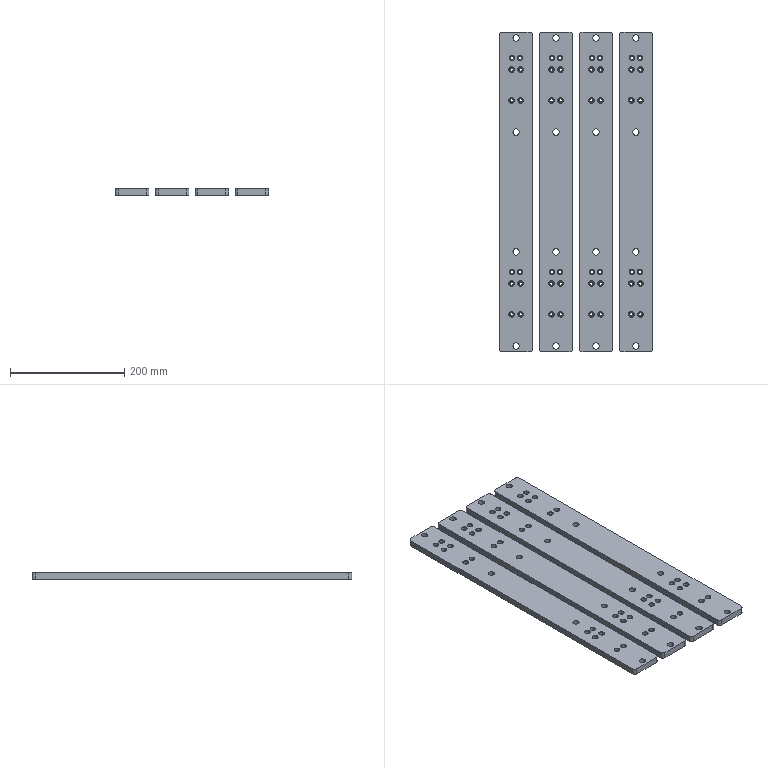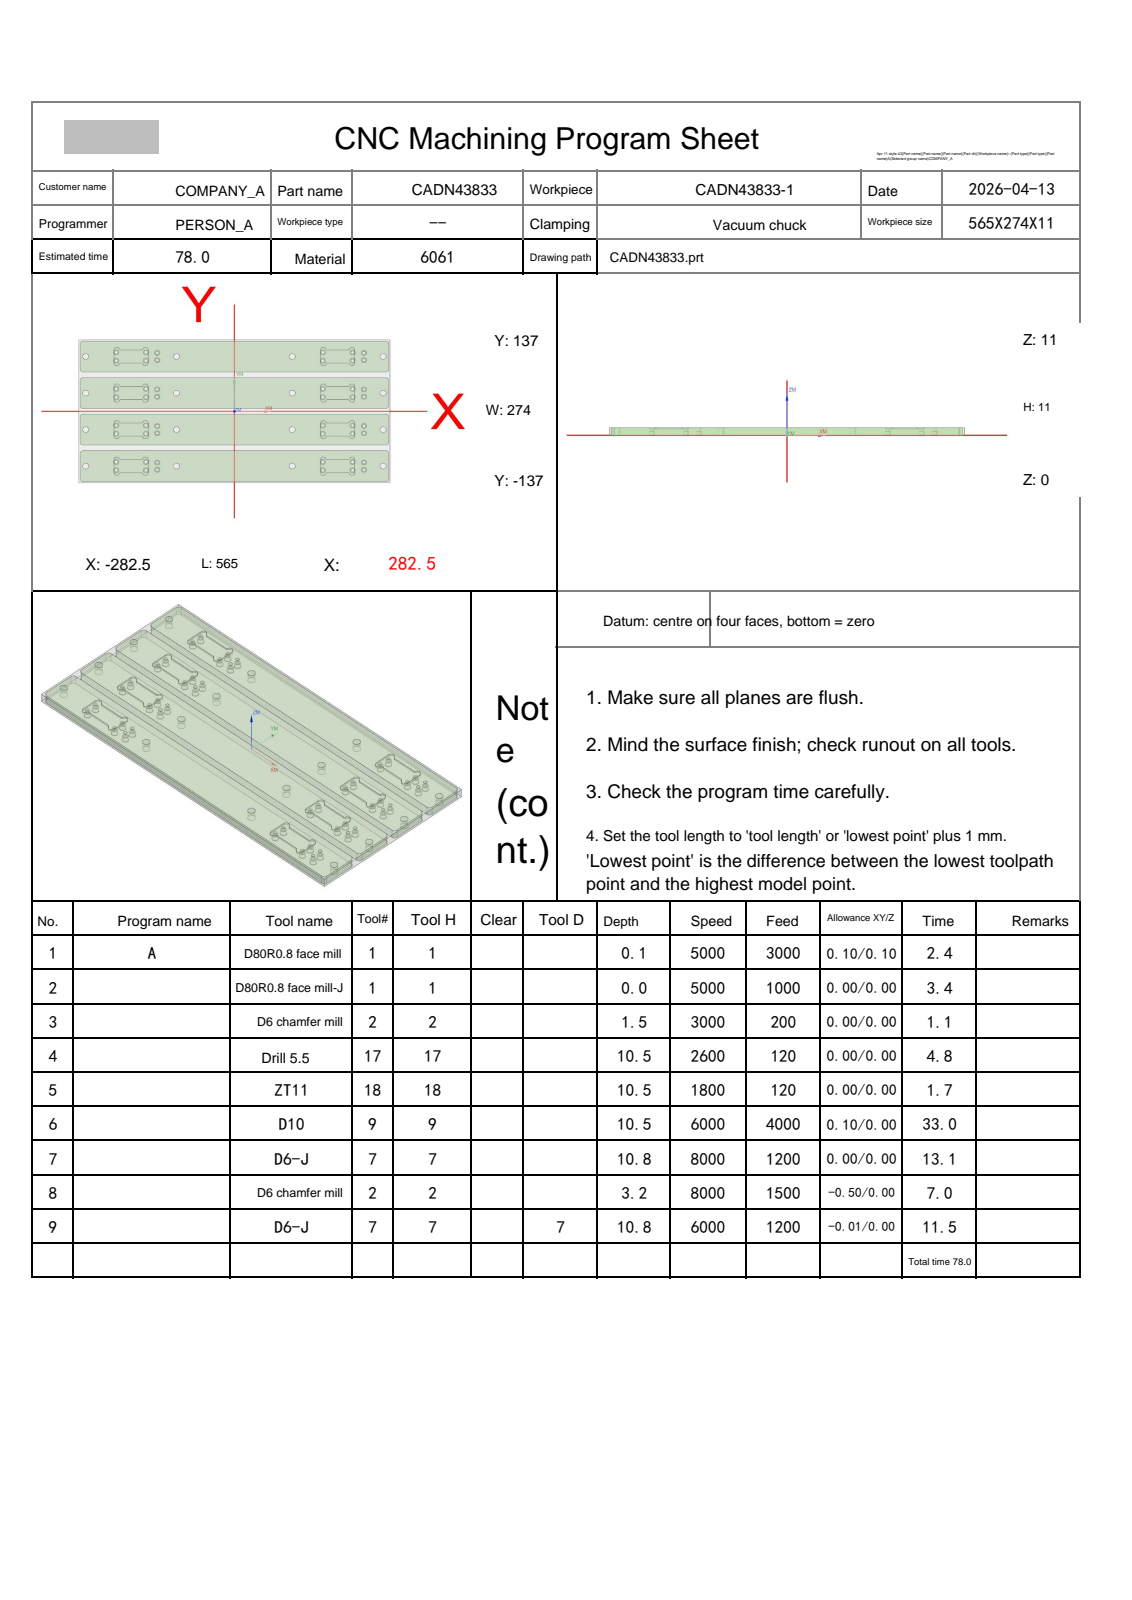NC program | NX | posted by the shop | part box 269 x 560 x 11 mm
Lines 4511 to 6644 of 6644, first 1747 of 2134 lines:
N8 T02 M06
(D6 chamfer mill  D=6. R=0. H=02 ce=0.00 di=0.00)
G00 G90 G54 X.386 Y74.373 M03 S8000
G43 H02 Z31.
M08
Z11.272
G01 Z9.8 F1350.
G03 X.1 Y74.573 I-1.286 J-1.532
G01 X.054 Y74.603
X0.0 Y74.6
X-275. F1500.
G02 X-280.9 Y80.5 I0.0 J5.9
G01 Y129.5
G02 X-275. Y135.4 I5.9 J0.0
G01 X275.
G02 X280.9 Y129.5 I0.0 J-5.9
G01 Y80.5
G02 X275. Y74.6 I-5.9 J0.0
G01 X0.0
X-.054 Y74.603
X-.1 Y74.573
G03 X-.386 Y74.373 I1. J-1.732
G01 Z11.272
G00 Z21.
X-269.6 Y109.399
Z11.323
G01 Z9.8 F1350.
G03 X-269.898 Y109.58 I-1.183 J-1.613
G01 X-269.946 Y109.606
X-270. Y109.6
G03 X-274.6 Y105. I0.0 J-4.6 F1500.
X-270. Y100.4 I4.6 J0.0
X-265.4 Y105. I0.0 J4.6
X-270. Y109.6 I-4.6 J0.0
G01 X-270.054 Y109.606
X-270.102 Y109.58
G03 X-270.4 Y109.399 I.885 J-1.794
G01 Z11.323
G00 Z21.
X-187.886 Y93.577
Z11.272
G01 Z9.8 F1350.
G03 X-187.6 Y93.377 I1.286 J1.532
G01 X-187.554 Y93.347
X-187.5 Y93.35
X-168.208 F1500.
G02 X-165.477 Y91.314 I0.0 J-2.85
G03 X-161.5 Y88.35 I3.977 J1.186
X-157.35 Y92.5 I0.0 J4.15
G01 Y117.5
G03 X-161.5 Y121.65 I-4.15 J0.0
X-165.477 Y118.686 I0.0 J-4.15
G02 X-168.208 Y116.65 I-2.731 J.814
G01 X-206.792
G02 X-209.523 Y118.686 I0.0 J2.85
G03 X-213.5 Y121.65 I-3.977 J-1.186
X-217.65 Y117.5 I0.0 J-4.15
G01 Y92.5
G03 X-213.5 Y88.35 I4.15 J0.0
X-209.523 Y91.314 I0.0 J4.15
G02 X-206.792 Y93.35 I2.731 J-.814
G01 X-187.5
X-187.446 Y93.347
X-187.4 Y93.377
G03 X-187.114 Y93.577 I-1. J1.732
G01 Z11.272
G00 Z21.
X-139.596 Y113.658
Z11.365
G01 Z9.8 F1350.
G03 X-139.898 Y113.832 I-1.147 J-1.638
G01 X-139.946 Y113.858
X-140. Y113.85
G03 X-141.85 Y112. I0.0 J-1.85 F1500.
X-140. Y110.15 I1.85 J0.0
X-138.15 Y112. I0.0 J1.85
X-139.679 Y113.822 I-1.85 J0.0
G01 X-140. Y113.85
X-140.054 Y113.858
X-140.102 Y113.832
G03 X-140.404 Y113.658 I.845 J-1.813
G01 Z11.365
G00 Z21.
X-139.596 Y99.658
Z11.365
G01 Z9.8 F1350.
G03 X-139.898 Y99.832 I-1.147 J-1.638
G01 X-139.946 Y99.858
X-140. Y99.85
G03 X-141.85 Y98. I0.0 J-1.85 F1500.
X-140. Y96.15 I1.85 J0.0
X-138.15 Y98. I0.0 J1.85
X-139.679 Y99.822 I-1.85 J0.0
G01 X-140. Y99.85
X-140.054 Y99.858
X-140.102 Y99.832
G03 X-140.404 Y99.658 I.845 J-1.813
G01 Z11.365
G00 Z21.
X-104.6 Y109.399
Z11.323
G01 Z9.8 F1350.
G03 X-104.898 Y109.58 I-1.183 J-1.613
G01 X-104.946 Y109.606
X-105. Y109.6
G03 X-109.6 Y105. I0.0 J-4.6 F1500.
X-105. Y100.4 I4.6 J0.0
X-100.4 Y105. I0.0 J4.6
X-105. Y109.6 I-4.6 J0.0
G01 X-105.054 Y109.606
X-105.102 Y109.58
G03 X-105.4 Y109.399 I.885 J-1.794
G01 Z11.323
G00 Z21.
X105.4
Z11.323
G01 Z9.8 F1350.
G03 X105.102 Y109.58 I-1.183 J-1.613
G01 X105.054 Y109.606
X105. Y109.6
G03 X100.4 Y105. I0.0 J-4.6 F1500.
X105. Y100.4 I4.6 J0.0
X109.6 Y105. I0.0 J4.6
X105. Y109.6 I-4.6 J0.0
G01 X104.946 Y109.606
X104.898 Y109.58
G03 X104.6 Y109.399 I.885 J-1.794
G01 Z11.323
G00 Z21.
X187.114 Y93.577
Z11.272
G01 Z9.8 F1350.
G03 X187.4 Y93.377 I1.286 J1.532
G01 X187.446 Y93.347
X187.5 Y93.35
X206.792 F1500.
G02 X209.523 Y91.314 I0.0 J-2.85
G03 X213.5 Y88.35 I3.977 J1.186
X217.65 Y92.5 I0.0 J4.15
G01 Y117.5
G03 X213.5 Y121.65 I-4.15 J0.0
X209.523 Y118.686 I0.0 J-4.15
G02 X206.792 Y116.65 I-2.731 J.814
G01 X168.208
G02 X165.477 Y118.686 I0.0 J2.85
G03 X161.5 Y121.65 I-3.977 J-1.186
X157.35 Y117.5 I0.0 J-4.15
G01 Y92.5
G03 X161.5 Y88.35 I4.15 J0.0
X165.477 Y91.314 I0.0 J4.15
G02 X168.208 Y93.35 I2.731 J-.814
G01 X187.5
X187.554 Y93.347
X187.6 Y93.377
G03 X187.886 Y93.577 I-1. J1.732
G01 Z11.272
G00 Z21.
X235.404 Y99.658
Z11.365
G01 Z9.8 F1350.
G03 X235.102 Y99.832 I-1.147 J-1.638
G01 X235.054 Y99.858
X235. Y99.85
G03 X233.15 Y98. I0.0 J-1.85 F1500.
X235. Y96.15 I1.85 J0.0
X236.85 Y98. I0.0 J1.85
X235.321 Y99.822 I-1.85 J0.0
G01 X235. Y99.85
X234.946 Y99.858
X234.898 Y99.832
G03 X234.596 Y99.658 I.845 J-1.813
G01 Z11.365
G00 Z21.
X235.404 Y113.658
Z11.365
G01 Z9.8 F1350.
G03 X235.102 Y113.832 I-1.147 J-1.638
G01 X235.054 Y113.858
X235. Y113.85
G03 X233.15 Y112. I0.0 J-1.85 F1500.
X235. Y110.15 I1.85 J0.0
X236.85 Y112. I0.0 J1.85
X235.321 Y113.822 I-1.85 J0.0
G01 X235. Y113.85
X234.946 Y113.858
X234.898 Y113.832
G03 X234.596 Y113.658 I.845 J-1.813
G01 Z11.365
G00 Z21.
X270.4 Y109.399
Z11.323
G01 Z9.8 F1350.
G03 X270.102 Y109.58 I-1.183 J-1.613
G01 X270.054 Y109.606
X270. Y109.6
G03 X265.4 Y105. I0.0 J-4.6 F1500.
X270. Y100.4 I4.6 J0.0
X274.6 Y105. I0.0 J4.6
X270. Y109.6 I-4.6 J0.0
G01 X269.946 Y109.606
X269.898 Y109.58
G03 X269.6 Y109.399 I.885 J-1.794
G01 Z11.323
G00 Z21.
X.386 Y4.373
Z11.272
G01 Z9.8 F1350.
G03 X.1 Y4.573 I-1.286 J-1.532
G01 X.054 Y4.603
X0.0 Y4.6
X-275. F1500.
G02 X-280.9 Y10.5 I0.0 J5.9
G01 Y59.5
G02 X-275. Y65.4 I5.9 J0.0
G01 X275.
G02 X280.9 Y59.5 I0.0 J-5.9
G01 Y10.5
G02 X275. Y4.6 I-5.9 J0.0
G01 X0.0
X-.054 Y4.603
X-.1 Y4.573
G03 X-.386 Y4.373 I1. J-1.732
G01 Z11.272
G00 Z21.
X-269.6 Y39.399
Z11.323
G01 Z9.8 F1350.
G03 X-269.898 Y39.58 I-1.183 J-1.613
G01 X-269.946 Y39.606
X-270. Y39.6
G03 X-274.6 Y35. I0.0 J-4.6 F1500.
X-270. Y30.4 I4.6 J0.0
X-265.4 Y35. I0.0 J4.6
X-270. Y39.6 I-4.6 J0.0
G01 X-270.054 Y39.606
X-270.102 Y39.58
G03 X-270.4 Y39.399 I.885 J-1.794
G01 Z11.323
G00 Z21.
X-187.886 Y23.577
Z11.272
G01 Z9.8 F1350.
G03 X-187.6 Y23.377 I1.286 J1.532
G01 X-187.554 Y23.347
X-187.5 Y23.35
X-168.208 F1500.
G02 X-165.477 Y21.314 I0.0 J-2.85
G03 X-161.5 Y18.35 I3.977 J1.186
X-157.35 Y22.5 I0.0 J4.15
G01 Y47.5
G03 X-161.5 Y51.65 I-4.15 J0.0
X-165.477 Y48.686 I0.0 J-4.15
G02 X-168.208 Y46.65 I-2.731 J.814
G01 X-206.792
G02 X-209.523 Y48.686 I0.0 J2.85
G03 X-213.5 Y51.65 I-3.977 J-1.186
X-217.65 Y47.5 I0.0 J-4.15
G01 Y22.5
G03 X-213.5 Y18.35 I4.15 J0.0
X-209.523 Y21.314 I0.0 J4.15
G02 X-206.792 Y23.35 I2.731 J-.814
G01 X-187.5
X-187.446 Y23.347
X-187.4 Y23.377
G03 X-187.114 Y23.577 I-1. J1.732
G01 Z11.272
G00 Z21.
X-139.596 Y29.658
Z11.365
G01 Z9.8 F1350.
G03 X-139.898 Y29.832 I-1.147 J-1.638
G01 X-139.946 Y29.858
X-140. Y29.85
G03 X-141.85 Y28. I0.0 J-1.85 F1500.
X-140. Y26.15 I1.85 J0.0
X-138.15 Y28. I0.0 J1.85
X-139.679 Y29.822 I-1.85 J0.0
G01 X-140. Y29.85
X-140.054 Y29.858
X-140.102 Y29.832
G03 X-140.404 Y29.658 I.845 J-1.813
G01 Z11.365
G00 Z21.
X-139.596 Y43.658
Z11.365
G01 Z9.8 F1350.
G03 X-139.898 Y43.832 I-1.147 J-1.638
G01 X-139.946 Y43.858
X-140. Y43.85
G03 X-141.85 Y42. I0.0 J-1.85 F1500.
X-140. Y40.15 I1.85 J0.0
X-138.15 Y42. I0.0 J1.85
X-139.679 Y43.822 I-1.85 J0.0
G01 X-140. Y43.85
X-140.054 Y43.858
X-140.102 Y43.832
G03 X-140.404 Y43.658 I.845 J-1.813
G01 Z11.365
G00 Z21.
X-104.6 Y39.399
Z11.323
G01 Z9.8 F1350.
G03 X-104.898 Y39.58 I-1.183 J-1.613
G01 X-104.946 Y39.606
X-105. Y39.6
G03 X-109.6 Y35. I0.0 J-4.6 F1500.
X-105. Y30.4 I4.6 J0.0
X-100.4 Y35. I0.0 J4.6
X-105. Y39.6 I-4.6 J0.0
G01 X-105.054 Y39.606
X-105.102 Y39.58
G03 X-105.4 Y39.399 I.885 J-1.794
G01 Z11.323
G00 Z21.
X105.4
Z11.323
G01 Z9.8 F1350.
G03 X105.102 Y39.58 I-1.183 J-1.613
G01 X105.054 Y39.606
X105. Y39.6
G03 X100.4 Y35. I0.0 J-4.6 F1500.
X105. Y30.4 I4.6 J0.0
X109.6 Y35. I0.0 J4.6
X105. Y39.6 I-4.6 J0.0
G01 X104.946 Y39.606
X104.898 Y39.58
G03 X104.6 Y39.399 I.885 J-1.794
G01 Z11.323
G00 Z21.
X187.114 Y23.577
Z11.272
G01 Z9.8 F1350.
G03 X187.4 Y23.377 I1.286 J1.532
G01 X187.446 Y23.347
X187.5 Y23.35
X206.792 F1500.
G02 X209.523 Y21.314 I0.0 J-2.85
G03 X213.5 Y18.35 I3.977 J1.186
X217.65 Y22.5 I0.0 J4.15
G01 Y47.5
G03 X213.5 Y51.65 I-4.15 J0.0
X209.523 Y48.686 I0.0 J-4.15
G02 X206.792 Y46.65 I-2.731 J.814
G01 X168.208
G02 X165.477 Y48.686 I0.0 J2.85
G03 X161.5 Y51.65 I-3.977 J-1.186
X157.35 Y47.5 I0.0 J-4.15
G01 Y22.5
G03 X161.5 Y18.35 I4.15 J0.0
X165.477 Y21.314 I0.0 J4.15
G02 X168.208 Y23.35 I2.731 J-.814
G01 X187.5
X187.554 Y23.347
X187.6 Y23.377
G03 X187.886 Y23.577 I-1. J1.732
G01 Z11.272
G00 Z21.
X235.404 Y43.658
Z11.365
G01 Z9.8 F1350.
G03 X235.102 Y43.832 I-1.147 J-1.638
G01 X235.054 Y43.858
X235. Y43.85
G03 X233.15 Y42. I0.0 J-1.85 F1500.
X235. Y40.15 I1.85 J0.0
X236.85 Y42. I0.0 J1.85
X235.321 Y43.822 I-1.85 J0.0
G01 X235. Y43.85
X234.946 Y43.858
X234.898 Y43.832
G03 X234.596 Y43.658 I.845 J-1.813
G01 Z11.365
G00 Z21.
X235.404 Y29.658
Z11.365
G01 Z9.8 F1350.
G03 X235.102 Y29.832 I-1.147 J-1.638
G01 X235.054 Y29.858
X235. Y29.85
G03 X233.15 Y28. I0.0 J-1.85 F1500.
X235. Y26.15 I1.85 J0.0
X236.85 Y28. I0.0 J1.85
X235.321 Y29.822 I-1.85 J0.0
G01 X235. Y29.85
X234.946 Y29.858
X234.898 Y29.832
G03 X234.596 Y29.658 I.845 J-1.813
G01 Z11.365
G00 Z21.
X270.4 Y39.399
Z11.323
G01 Z9.8 F1350.
G03 X270.102 Y39.58 I-1.183 J-1.613
G01 X270.054 Y39.606
X270. Y39.6
G03 X265.4 Y35. I0.0 J-4.6 F1500.
X270. Y30.4 I4.6 J0.0
X274.6 Y35. I0.0 J4.6
X270. Y39.6 I-4.6 J0.0
G01 X269.946 Y39.606
X269.898 Y39.58
G03 X269.6 Y39.399 I.885 J-1.794
G01 Z11.323
G00 Z21.
X.386 Y-65.627
Z11.272
G01 Z9.8 F1350.
G03 X.1 Y-65.427 I-1.286 J-1.532
G01 X.054 Y-65.397
X0.0 Y-65.4
X-275. F1500.
G02 X-280.9 Y-59.5 I0.0 J5.9
G01 Y-10.5
G02 X-275. Y-4.6 I5.9 J0.0
G01 X275.
G02 X280.9 Y-10.5 I0.0 J-5.9
G01 Y-59.5
G02 X275. Y-65.4 I-5.9 J0.0
G01 X0.0
X-.054 Y-65.397
X-.1 Y-65.427
G03 X-.386 Y-65.627 I1. J-1.732
G01 Z11.272
G00 Z21.
X-269.6 Y-30.601
Z11.323
G01 Z9.8 F1350.
G03 X-269.898 Y-30.42 I-1.183 J-1.613
G01 X-269.946 Y-30.394
X-270. Y-30.4
G03 X-274.6 Y-35. I0.0 J-4.6 F1500.
X-270. Y-39.6 I4.6 J0.0
X-265.4 Y-35. I0.0 J4.6
X-270. Y-30.4 I-4.6 J0.0
G01 X-270.054 Y-30.394
X-270.102 Y-30.42
G03 X-270.4 Y-30.601 I.885 J-1.794
G01 Z11.323
G00 Z21.
X-187.886 Y-46.423
Z11.272
G01 Z9.8 F1350.
G03 X-187.6 Y-46.623 I1.286 J1.532
G01 X-187.554 Y-46.653
X-187.5 Y-46.65
X-168.208 F1500.
G02 X-165.477 Y-48.686 I0.0 J-2.85
G03 X-161.5 Y-51.65 I3.977 J1.186
X-157.35 Y-47.5 I0.0 J4.15
G01 Y-22.5
G03 X-161.5 Y-18.35 I-4.15 J0.0
X-165.477 Y-21.314 I0.0 J-4.15
G02 X-168.208 Y-23.35 I-2.731 J.814
G01 X-206.792
G02 X-209.523 Y-21.314 I0.0 J2.85
G03 X-213.5 Y-18.35 I-3.977 J-1.186
X-217.65 Y-22.5 I0.0 J-4.15
G01 Y-47.5
G03 X-213.5 Y-51.65 I4.15 J0.0
X-209.523 Y-48.686 I0.0 J4.15
G02 X-206.792 Y-46.65 I2.731 J-.814
G01 X-187.5
X-187.446 Y-46.653
X-187.4 Y-46.623
G03 X-187.114 Y-46.423 I-1. J1.732
G01 Z11.272
G00 Z21.
X-139.596 Y-40.342
Z11.365
G01 Z9.8 F1350.
G03 X-139.898 Y-40.168 I-1.147 J-1.638
G01 X-139.946 Y-40.142
X-140. Y-40.15
G03 X-141.85 Y-42. I0.0 J-1.85 F1500.
X-140. Y-43.85 I1.85 J0.0
X-138.15 Y-42. I0.0 J1.85
X-139.679 Y-40.178 I-1.85 J0.0
G01 X-140. Y-40.15
X-140.054 Y-40.142
X-140.102 Y-40.168
G03 X-140.404 Y-40.342 I.845 J-1.813
G01 Z11.365
G00 Z21.
X-139.596 Y-26.342
Z11.365
G01 Z9.8 F1350.
G03 X-139.898 Y-26.168 I-1.147 J-1.638
G01 X-139.946 Y-26.142
X-140. Y-26.15
G03 X-141.85 Y-28. I0.0 J-1.85 F1500.
X-140. Y-29.85 I1.85 J0.0
X-138.15 Y-28. I0.0 J1.85
X-139.679 Y-26.178 I-1.85 J0.0
G01 X-140. Y-26.15
X-140.054 Y-26.142
X-140.102 Y-26.168
G03 X-140.404 Y-26.342 I.845 J-1.813
G01 Z11.365
G00 Z21.
X-104.6 Y-30.601
Z11.323
G01 Z9.8 F1350.
G03 X-104.898 Y-30.42 I-1.183 J-1.613
G01 X-104.946 Y-30.394
X-105. Y-30.4
G03 X-109.6 Y-35. I0.0 J-4.6 F1500.
X-105. Y-39.6 I4.6 J0.0
X-100.4 Y-35. I0.0 J4.6
X-105. Y-30.4 I-4.6 J0.0
G01 X-105.054 Y-30.394
X-105.102 Y-30.42
G03 X-105.4 Y-30.601 I.885 J-1.794
G01 Z11.323
G00 Z21.
X105.4
Z11.323
G01 Z9.8 F1350.
G03 X105.102 Y-30.42 I-1.183 J-1.613
G01 X105.054 Y-30.394
X105. Y-30.4
G03 X100.4 Y-35. I0.0 J-4.6 F1500.
X105. Y-39.6 I4.6 J0.0
X109.6 Y-35. I0.0 J4.6
X105. Y-30.4 I-4.6 J0.0
G01 X104.946 Y-30.394
X104.898 Y-30.42
G03 X104.6 Y-30.601 I.885 J-1.794
G01 Z11.323
G00 Z21.
X187.114 Y-46.423
Z11.272
G01 Z9.8 F1350.
G03 X187.4 Y-46.623 I1.286 J1.532
G01 X187.446 Y-46.653
X187.5 Y-46.65
X206.792 F1500.
G02 X209.523 Y-48.686 I0.0 J-2.85
G03 X213.5 Y-51.65 I3.977 J1.186
X217.65 Y-47.5 I0.0 J4.15
G01 Y-22.5
G03 X213.5 Y-18.35 I-4.15 J0.0
X209.523 Y-21.314 I0.0 J-4.15
G02 X206.792 Y-23.35 I-2.731 J.814
G01 X168.208
G02 X165.477 Y-21.314 I0.0 J2.85
G03 X161.5 Y-18.35 I-3.977 J-1.186
X157.35 Y-22.5 I0.0 J-4.15
G01 Y-47.5
G03 X161.5 Y-51.65 I4.15 J0.0
X165.477 Y-48.686 I0.0 J4.15
G02 X168.208 Y-46.65 I2.731 J-.814
G01 X187.5
X187.554 Y-46.653
X187.6 Y-46.623
G03 X187.886 Y-46.423 I-1. J1.732
G01 Z11.272
G00 Z21.
X235.404 Y-40.342
Z11.365
G01 Z9.8 F1350.
G03 X235.102 Y-40.168 I-1.147 J-1.638
G01 X235.054 Y-40.142
X235. Y-40.15
G03 X233.15 Y-42. I0.0 J-1.85 F1500.
X235. Y-43.85 I1.85 J0.0
X236.85 Y-42. I0.0 J1.85
X235.321 Y-40.178 I-1.85 J0.0
G01 X235. Y-40.15
X234.946 Y-40.142
X234.898 Y-40.168
G03 X234.596 Y-40.342 I.845 J-1.813
G01 Z11.365
G00 Z21.
X235.404 Y-26.342
Z11.365
G01 Z9.8 F1350.
G03 X235.102 Y-26.168 I-1.147 J-1.638
G01 X235.054 Y-26.142
X235. Y-26.15
G03 X233.15 Y-28. I0.0 J-1.85 F1500.
X235. Y-29.85 I1.85 J0.0
X236.85 Y-28. I0.0 J1.85
X235.321 Y-26.178 I-1.85 J0.0
G01 X235. Y-26.15
X234.946 Y-26.142
X234.898 Y-26.168
G03 X234.596 Y-26.342 I.845 J-1.813
G01 Z11.365
G00 Z21.
X270.4 Y-30.601
Z11.323
G01 Z9.8 F1350.
G03 X270.102 Y-30.42 I-1.183 J-1.613
G01 X270.054 Y-30.394
X270. Y-30.4
G03 X265.4 Y-35. I0.0 J-4.6 F1500.
X270. Y-39.6 I4.6 J0.0
X274.6 Y-35. I0.0 J4.6
X270. Y-30.4 I-4.6 J0.0
G01 X269.946 Y-30.394
X269.898 Y-30.42
G03 X269.6 Y-30.601 I.885 J-1.794
G01 Z11.323
G00 Z21.
X.386 Y-135.627
Z11.272
G01 Z9.8 F1350.
G03 X.1 Y-135.427 I-1.286 J-1.532
G01 X.054 Y-135.397
X0.0 Y-135.4
X-275. F1500.
G02 X-280.9 Y-129.5 I0.0 J5.9
G01 Y-80.5
G02 X-275. Y-74.6 I5.9 J0.0
G01 X275.
G02 X280.9 Y-80.5 I0.0 J-5.9
G01 Y-129.5
G02 X275. Y-135.4 I-5.9 J0.0
G01 X0.0
X-.054 Y-135.397
X-.1 Y-135.427
G03 X-.386 Y-135.627 I1. J-1.732
G01 Z11.272
G00 Z21.
X-269.6 Y-100.601
Z11.323
G01 Z9.8 F1350.
G03 X-269.898 Y-100.42 I-1.183 J-1.613
G01 X-269.946 Y-100.394
X-270. Y-100.4
G03 X-274.6 Y-105. I0.0 J-4.6 F1500.
X-270. Y-109.6 I4.6 J0.0
X-265.4 Y-105. I0.0 J4.6
X-270. Y-100.4 I-4.6 J0.0
G01 X-270.054 Y-100.394
X-270.102 Y-100.42
G03 X-270.4 Y-100.601 I.885 J-1.794
G01 Z11.323
G00 Z21.
X-187.886 Y-116.423
Z11.272
G01 Z9.8 F1350.
G03 X-187.6 Y-116.623 I1.286 J1.532
G01 X-187.554 Y-116.653
X-187.5 Y-116.65
X-168.208 F1500.
G02 X-165.477 Y-118.686 I0.0 J-2.85
G03 X-161.5 Y-121.65 I3.977 J1.186
X-157.35 Y-117.5 I0.0 J4.15
G01 Y-92.5
G03 X-161.5 Y-88.35 I-4.15 J0.0
X-165.477 Y-91.314 I0.0 J-4.15
G02 X-168.208 Y-93.35 I-2.731 J.814
G01 X-206.792
G02 X-209.523 Y-91.314 I0.0 J2.85
G03 X-213.5 Y-88.35 I-3.977 J-1.186
X-217.65 Y-92.5 I0.0 J-4.15
G01 Y-117.5
G03 X-213.5 Y-121.65 I4.15 J0.0
X-209.523 Y-118.686 I0.0 J4.15
G02 X-206.792 Y-116.65 I2.731 J-.814
G01 X-187.5
X-187.446 Y-116.653
X-187.4 Y-116.623
G03 X-187.114 Y-116.423 I-1. J1.732
G01 Z11.272
G00 Z21.
X-139.596 Y-96.342
Z11.365
G01 Z9.8 F1350.
G03 X-139.898 Y-96.168 I-1.147 J-1.638
G01 X-139.946 Y-96.142
X-140. Y-96.15
G03 X-141.85 Y-98. I0.0 J-1.85 F1500.
X-140. Y-99.85 I1.85 J0.0
X-138.15 Y-98. I0.0 J1.85
X-139.679 Y-96.178 I-1.85 J0.0
G01 X-140. Y-96.15
X-140.054 Y-96.142
X-140.102 Y-96.168
G03 X-140.404 Y-96.342 I.845 J-1.813
G01 Z11.365
G00 Z21.
X-139.596 Y-110.342
Z11.365
G01 Z9.8 F1350.
G03 X-139.898 Y-110.168 I-1.147 J-1.638
G01 X-139.946 Y-110.142
X-140. Y-110.15
G03 X-141.85 Y-112. I0.0 J-1.85 F1500.
X-140. Y-113.85 I1.85 J0.0
X-138.15 Y-112. I0.0 J1.85
X-139.679 Y-110.178 I-1.85 J0.0
G01 X-140. Y-110.15
X-140.054 Y-110.142
X-140.102 Y-110.168
G03 X-140.404 Y-110.342 I.845 J-1.813
G01 Z11.365
G00 Z21.
X-104.6 Y-100.601
Z11.323
G01 Z9.8 F1350.
G03 X-104.898 Y-100.42 I-1.183 J-1.613
G01 X-104.946 Y-100.394
X-105. Y-100.4
G03 X-109.6 Y-105. I0.0 J-4.6 F1500.
X-105. Y-109.6 I4.6 J0.0
X-100.4 Y-105. I0.0 J4.6
X-105. Y-100.4 I-4.6 J0.0
G01 X-105.054 Y-100.394
X-105.102 Y-100.42
G03 X-105.4 Y-100.601 I.885 J-1.794
G01 Z11.323
G00 Z21.
X105.4
Z11.323
G01 Z9.8 F1350.
G03 X105.102 Y-100.42 I-1.183 J-1.613
G01 X105.054 Y-100.394
X105. Y-100.4
G03 X100.4 Y-105. I0.0 J-4.6 F1500.
X105. Y-109.6 I4.6 J0.0
X109.6 Y-105. I0.0 J4.6
X105. Y-100.4 I-4.6 J0.0
G01 X104.946 Y-100.394
X104.898 Y-100.42
G03 X104.6 Y-100.601 I.885 J-1.794
G01 Z11.323
G00 Z21.
X187.114 Y-116.423
Z11.272
G01 Z9.8 F1350.
G03 X187.4 Y-116.623 I1.286 J1.532
G01 X187.446 Y-116.653
X187.5 Y-116.65
X206.792 F1500.
G02 X209.523 Y-118.686 I0.0 J-2.85
G03 X213.5 Y-121.65 I3.977 J1.186
X217.65 Y-117.5 I0.0 J4.15
G01 Y-92.5
G03 X213.5 Y-88.35 I-4.15 J0.0
X209.523 Y-91.314 I0.0 J-4.15
G02 X206.792 Y-93.35 I-2.731 J.814
G01 X168.208
G02 X165.477 Y-91.314 I0.0 J2.85
G03 X161.5 Y-88.35 I-3.977 J-1.186
X157.35 Y-92.5 I0.0 J-4.15
G01 Y-117.5
G03 X161.5 Y-121.65 I4.15 J0.0
X165.477 Y-118.686 I0.0 J4.15
G02 X168.208 Y-116.65 I2.731 J-.814
G01 X187.5
X187.554 Y-116.653
X187.6 Y-116.623
G03 X187.886 Y-116.423 I-1. J1.732
G01 Z11.272
G00 Z21.
X235.404 Y-96.342
Z11.365
G01 Z9.8 F1350.
G03 X235.102 Y-96.168 I-1.147 J-1.638
G01 X235.054 Y-96.142
X235. Y-96.15
G03 X233.15 Y-98. I0.0 J-1.85 F1500.
X235. Y-99.85 I1.85 J0.0
X236.85 Y-98. I0.0 J1.85
X235.321 Y-96.178 I-1.85 J0.0
G01 X235. Y-96.15
X234.946 Y-96.142
X234.898 Y-96.168
G03 X234.596 Y-96.342 I.845 J-1.813
G01 Z11.365
G00 Z21.
X235.404 Y-110.342
Z11.365
G01 Z9.8 F1350.
G03 X235.102 Y-110.168 I-1.147 J-1.638
G01 X235.054 Y-110.142
X235. Y-110.15
G03 X233.15 Y-112. I0.0 J-1.85 F1500.
X235. Y-113.85 I1.85 J0.0
X236.85 Y-112. I0.0 J1.85
X235.321 Y-110.178 I-1.85 J0.0
G01 X235. Y-110.15
X234.946 Y-110.142
X234.898 Y-110.168
G03 X234.596 Y-110.342 I.845 J-1.813
G01 Z11.365
G00 Z21.
X270.4 Y-100.601
Z11.323
G01 Z9.8 F1350.
G03 X270.102 Y-100.42 I-1.183 J-1.613
G01 X270.054 Y-100.394
X270. Y-100.4
G03 X265.4 Y-105. I0.0 J-4.6 F1500.
X270. Y-109.6 I4.6 J0.0
X274.6 Y-105. I0.0 J4.6
X270. Y-100.4 I-4.6 J0.0
G01 X269.946 Y-100.394
X269.898 Y-100.42
G03 X269.6 Y-100.601 I.885 J-1.794
G01 Z11.323
G00 Z21.
X215.376 Y-111.456
Z9.428
G01 Z7.8 F1350.
X215.328 Y-111.364
X215.305 Y-111.343
X215.188 Y-111.283 F1500.
G03 X214.5 Y-111.15 I-.688 J-1.717
X212.65 Y-113. I0.0 J-1.85
X214.5 Y-114.85 I1.85 J0.0
G01 X214.821 Y-114.822
X215.133 Y-114.738
X215.279 Y-114.67
X215.305 Y-114.654
X215.328 Y-114.648
X215.333 Y-114.624
X215.373 Y-114.565
X215.388 Y-114.496
Z9.398
G00 Z21.
X215.376 Y-95.456
Z9.428
G01 Z7.8 F1350.
X215.328 Y-95.364
X215.305 Y-95.343
X215.188 Y-95.283 F1500.
G03 X214.5 Y-95.15 I-.688 J-1.717
X212.65 Y-97. I0.0 J-1.85
X214.5 Y-98.85 I1.85 J0.0
X215.133 Y-98.738 I0.0 J1.85
G01 X215.279 Y-98.67
X215.305 Y-98.654
X215.328 Y-98.648
X215.333 Y-98.624
X215.373 Y-98.565
X215.388 Y-98.496
Z9.398
G00 Z21.
X159.62 Y-98.523
Z9.417
G01 Z7.8 F1350.
X159.643 Y-98.59
X159.689 Y-98.644
X159.697 Y-98.667
X159.721 Y-98.67
X159.867 Y-98.738 F1500.
G03 X160.5 Y-98.85 I.633 J1.738
X162.35 Y-97. I0.0 J1.85
X160.5 Y-95.15 I-1.85 J0.0
X159.812 Y-95.283 I0.0 J-1.85
G01 X159.695 Y-95.343
X159.672 Y-95.364
X159.624 Y-95.456
Z9.428
G00 Z21.
X159.62 Y-114.523
Z9.417
G01 Z7.8 F1350.
X159.643 Y-114.59
X159.689 Y-114.644
X159.697 Y-114.667
X159.721 Y-114.67
X159.867 Y-114.738 F1500.
X160.179 Y-114.822
X160.5 Y-114.85
G03 X162.35 Y-113. I0.0 J1.85
X160.5 Y-111.15 I-1.85 J0.0
X159.812 Y-111.283 I0.0 J-1.85
G01 X159.695 Y-111.343
X159.672 Y-111.364
X159.624 Y-111.456
Z9.428
G00 Z21.
X215.376 Y-41.456
Z9.428
G01 Z7.8 F1350.
X215.328 Y-41.364
X215.305 Y-41.343
X215.188 Y-41.283 F1500.
G03 X214.5 Y-41.15 I-.688 J-1.717
X212.65 Y-43. I0.0 J-1.85
X214.5 Y-44.85 I1.85 J0.0
G01 X214.821 Y-44.822
X215.133 Y-44.738
X215.279 Y-44.67
X215.305 Y-44.654
X215.328 Y-44.648
X215.333 Y-44.624
X215.373 Y-44.565
X215.388 Y-44.496
Z9.398
G00 Z21.
X215.376 Y-25.456
Z9.428
G01 Z7.8 F1350.
X215.328 Y-25.364
X215.305 Y-25.343
X215.188 Y-25.283 F1500.
G03 X214.5 Y-25.15 I-.688 J-1.717
X212.65 Y-27. I0.0 J-1.85
X214.5 Y-28.85 I1.85 J0.0
X215.133 Y-28.738 I0.0 J1.85
G01 X215.279 Y-28.67
X215.305 Y-28.654
X215.328 Y-28.648
X215.333 Y-28.624
X215.373 Y-28.565
X215.388 Y-28.496
Z9.398
G00 Z21.
X159.62 Y-28.523
Z9.417
G01 Z7.8 F1350.
X159.643 Y-28.59
X159.689 Y-28.644
X159.697 Y-28.667
X159.721 Y-28.67
X159.867 Y-28.738 F1500.
G03 X160.5 Y-28.85 I.633 J1.738
X162.35 Y-27. I0.0 J1.85
X160.5 Y-25.15 I-1.85 J0.0
X159.812 Y-25.283 I0.0 J-1.85
G01 X159.695 Y-25.343
X159.672 Y-25.364
X159.624 Y-25.456
Z9.428
G00 Z21.
X159.62 Y-44.523
Z9.417
G01 Z7.8 F1350.
X159.643 Y-44.59
X159.689 Y-44.644
X159.697 Y-44.667
X159.721 Y-44.67
X159.867 Y-44.738 F1500.
X160.179 Y-44.822
X160.5 Y-44.85
G03 X162.35 Y-43. I0.0 J1.85
X160.5 Y-41.15 I-1.85 J0.0
X159.812 Y-41.283 I0.0 J-1.85
G01 X159.695 Y-41.343
X159.672 Y-41.364
X159.624 Y-41.456
Z9.428
G00 Z21.
X215.376 Y28.544
Z9.428
G01 Z7.8 F1350.
X215.328 Y28.636
X215.305 Y28.657
X215.188 Y28.717 F1500.
G03 X214.5 Y28.85 I-.688 J-1.717
X212.65 Y27. I0.0 J-1.85
X214.5 Y25.15 I1.85 J0.0
G01 X214.821 Y25.178
X215.133 Y25.262
X215.279 Y25.33
X215.305 Y25.346
X215.328 Y25.352
X215.333 Y25.376
X215.373 Y25.435
X215.388 Y25.504
Z9.398
G00 Z21.
X215.376 Y44.544
Z9.428
G01 Z7.8 F1350.
X215.328 Y44.636
X215.305 Y44.657
X215.188 Y44.717 F1500.
G03 X214.5 Y44.85 I-.688 J-1.717
X212.65 Y43. I0.0 J-1.85
X214.5 Y41.15 I1.85 J0.0
X215.133 Y41.262 I0.0 J1.85
G01 X215.279 Y41.33
X215.305 Y41.346
X215.328 Y41.352
X215.333 Y41.376
X215.373 Y41.435
X215.388 Y41.504
Z9.398
G00 Z21.
X159.62 Y41.477
Z9.417
G01 Z7.8 F1350.
X159.643 Y41.41
X159.689 Y41.356
X159.697 Y41.333
X159.721 Y41.33
X159.867 Y41.262 F1500.
G03 X160.5 Y41.15 I.633 J1.738
X162.35 Y43. I0.0 J1.85
X160.5 Y44.85 I-1.85 J0.0
X159.812 Y44.717 I0.0 J-1.85
G01 X159.695 Y44.657
X159.672 Y44.636
X159.624 Y44.544
Z9.428
G00 Z21.
X159.62 Y25.477
Z9.417
G01 Z7.8 F1350.
X159.643 Y25.41
X159.689 Y25.356
X159.697 Y25.333
X159.721 Y25.33
X159.867 Y25.262 F1500.
X160.179 Y25.178
X160.5 Y25.15
G03 X162.35 Y27. I0.0 J1.85
X160.5 Y28.85 I-1.85 J0.0
X159.812 Y28.717 I0.0 J-1.85
G01 X159.695 Y28.657
X159.672 Y28.636
X159.624 Y28.544
Z9.428
G00 Z21.
X215.376 Y98.544
Z9.428
G01 Z7.8 F1350.
X215.328 Y98.636
X215.305 Y98.657
X215.188 Y98.717 F1500.
G03 X214.5 Y98.85 I-.688 J-1.717
X212.65 Y97. I0.0 J-1.85
X214.5 Y95.15 I1.85 J0.0
G01 X214.821 Y95.178
X215.133 Y95.262
X215.279 Y95.33
X215.305 Y95.346
X215.328 Y95.352
X215.333 Y95.376
X215.373 Y95.435
X215.388 Y95.504
Z9.398
G00 Z21.
X215.376 Y114.544
Z9.428
G01 Z7.8 F1350.
X215.328 Y114.636
X215.305 Y114.657
X215.188 Y114.717 F1500.
G03 X214.5 Y114.85 I-.688 J-1.717
X212.65 Y113. I0.0 J-1.85
X214.5 Y111.15 I1.85 J0.0
X215.133 Y111.262 I0.0 J1.85
G01 X215.279 Y111.33
X215.305 Y111.346
X215.328 Y111.352
X215.333 Y111.376
X215.373 Y111.435
X215.388 Y111.504
Z9.398
G00 Z21.
X159.62 Y111.477
Z9.417
G01 Z7.8 F1350.
X159.643 Y111.41
X159.689 Y111.356
X159.697 Y111.333
X159.721 Y111.33
X159.867 Y111.262 F1500.
G03 X160.5 Y111.15 I.633 J1.738
X162.35 Y113. I0.0 J1.85
X160.5 Y114.85 I-1.85 J0.0
X159.812 Y114.717 I0.0 J-1.85
G01 X159.695 Y114.657
X159.672 Y114.636
X159.624 Y114.544
Z9.428
G00 Z21.
X159.62 Y95.477
Z9.417
G01 Z7.8 F1350.
X159.643 Y95.41
X159.689 Y95.356
X159.697 Y95.333
X159.721 Y95.33
X159.867 Y95.262 F1500.
X160.179 Y95.178
X160.5 Y95.15
G03 X162.35 Y97. I0.0 J1.85
X160.5 Y98.85 I-1.85 J0.0
X159.812 Y98.717 I0.0 J-1.85
G01 X159.695 Y98.657
X159.672 Y98.636
X159.624 Y98.544
Z9.428
G00 Z21.
X-159.624
Z9.428
G01 Z7.8 F1350.
X-159.672 Y98.636
X-159.695 Y98.657
X-159.812 Y98.717 F1500.
G03 X-160.5 Y98.85 I-.688 J-1.717
X-162.35 Y97. I0.0 J-1.85
X-160.5 Y95.15 I1.85 J0.0
G01 X-160.179 Y95.178
X-159.867 Y95.262
X-159.721 Y95.33
X-159.695 Y95.346
X-159.672 Y95.352
X-159.667 Y95.376
X-159.627 Y95.435
X-159.612 Y95.504
Z9.398
G00 Z21.
X-159.624 Y114.544
Z9.428
G01 Z7.8 F1350.
X-159.672 Y114.636
X-159.695 Y114.657
X-159.812 Y114.717 F1500.
G03 X-160.5 Y114.85 I-.688 J-1.717
X-162.35 Y113. I0.0 J-1.85
X-160.5 Y111.15 I1.85 J0.0
X-159.867 Y111.262 I0.0 J1.85
G01 X-159.721 Y111.33
X-159.695 Y111.346
X-159.672 Y111.352
X-159.667 Y111.376
X-159.627 Y111.435
X-159.612 Y111.504
Z9.398
G00 Z21.
X-215.38 Y111.477
Z9.417
G01 Z7.8 F1350.
X-215.357 Y111.41
X-215.311 Y111.356
X-215.303 Y111.333
X-215.279 Y111.33
X-215.133 Y111.262 F1500.
G03 X-214.5 Y111.15 I.633 J1.738
X-212.65 Y113. I0.0 J1.85
X-214.5 Y114.85 I-1.85 J0.0
X-215.188 Y114.717 I0.0 J-1.85
G01 X-215.305 Y114.657
X-215.328 Y114.636
X-215.376 Y114.544
Z9.428
G00 Z21.
X-215.38 Y95.477
Z9.417
G01 Z7.8 F1350.
X-215.357 Y95.41
X-215.311 Y95.356
X-215.303 Y95.333
X-215.279 Y95.33
X-215.133 Y95.262 F1500.
X-214.821 Y95.178
X-214.5 Y95.15
G03 X-212.65 Y97. I0.0 J1.85
X-214.5 Y98.85 I-1.85 J0.0
X-215.188 Y98.717 I0.0 J-1.85
G01 X-215.305 Y98.657
X-215.328 Y98.636
X-215.376 Y98.544
Z9.428
G00 Z21.
X-159.624 Y28.544
Z9.428
G01 Z7.8 F1350.
X-159.672 Y28.636
X-159.695 Y28.657
X-159.812 Y28.717 F1500.
G03 X-160.5 Y28.85 I-.688 J-1.717
X-162.35 Y27. I0.0 J-1.85
X-160.5 Y25.15 I1.85 J0.0
G01 X-160.179 Y25.178
X-159.867 Y25.262
X-159.721 Y25.33
X-159.695 Y25.346
X-159.672 Y25.352
X-159.667 Y25.376
X-159.627 Y25.435
X-159.612 Y25.504
Z9.398
G00 Z21.
X-159.624 Y44.544
Z9.428
G01 Z7.8 F1350.
X-159.672 Y44.636
X-159.695 Y44.657
X-159.812 Y44.717 F1500.
G03 X-160.5 Y44.85 I-.688 J-1.717
X-162.35 Y43. I0.0 J-1.85
X-160.5 Y41.15 I1.85 J0.0
X-159.867 Y41.262 I0.0 J1.85
G01 X-159.721 Y41.33
X-159.695 Y41.346
X-159.672 Y41.352
X-159.667 Y41.376
X-159.627 Y41.435
X-159.612 Y41.504
Z9.398
G00 Z21.
X-215.38 Y41.477
Z9.417
G01 Z7.8 F1350.
X-215.357 Y41.41
X-215.311 Y41.356
X-215.303 Y41.333
X-215.279 Y41.33
X-215.133 Y41.262 F1500.
G03 X-214.5 Y41.15 I.633 J1.738
X-212.65 Y43. I0.0 J1.85
X-214.5 Y44.85 I-1.85 J0.0
X-215.188 Y44.717 I0.0 J-1.85
G01 X-215.305 Y44.657
X-215.328 Y44.636
X-215.376 Y44.544
Z9.428
G00 Z21.
X-215.38 Y25.477
Z9.417
G01 Z7.8 F1350.
X-215.357 Y25.41
X-215.311 Y25.356
X-215.303 Y25.333
X-215.279 Y25.33
X-215.133 Y25.262 F1500.
X-214.821 Y25.178
X-214.5 Y25.15
G03 X-212.65 Y27. I0.0 J1.85
X-214.5 Y28.85 I-1.85 J0.0
X-215.188 Y28.717 I0.0 J-1.85
G01 X-215.305 Y28.657
X-215.328 Y28.636
X-215.376 Y28.544
Z9.428
G00 Z21.
X-159.624 Y-41.456
Z9.428
G01 Z7.8 F1350.
X-159.672 Y-41.364
X-159.695 Y-41.343
X-159.812 Y-41.283 F1500.
G03 X-160.5 Y-41.15 I-.688 J-1.717
X-162.35 Y-43. I0.0 J-1.85
X-160.5 Y-44.85 I1.85 J0.0
G01 X-160.179 Y-44.822
X-159.867 Y-44.738
X-159.721 Y-44.67
X-159.695 Y-44.654
X-159.672 Y-44.648
X-159.667 Y-44.624
X-159.627 Y-44.565
X-159.612 Y-44.496
Z9.398
G00 Z21.
X-159.624 Y-25.456
Z9.428
G01 Z7.8 F1350.
X-159.672 Y-25.364
X-159.695 Y-25.343
X-159.812 Y-25.283 F1500.
G03 X-160.5 Y-25.15 I-.688 J-1.717
X-162.35 Y-27. I0.0 J-1.85
X-160.5 Y-28.85 I1.85 J0.0
X-159.867 Y-28.738 I0.0 J1.85
G01 X-159.721 Y-28.67
X-159.695 Y-28.654
X-159.672 Y-28.648
X-159.667 Y-28.624
X-159.627 Y-28.565
X-159.612 Y-28.496
Z9.398
G00 Z21.
X-215.38 Y-28.523
Z9.417
G01 Z7.8 F1350.
X-215.357 Y-28.59
X-215.311 Y-28.644
X-215.303 Y-28.667
X-215.279 Y-28.67
X-215.133 Y-28.738 F1500.
G03 X-214.5 Y-28.85 I.633 J1.738
X-212.65 Y-27. I0.0 J1.85
X-214.5 Y-25.15 I-1.85 J0.0
X-215.188 Y-25.283 I0.0 J-1.85
G01 X-215.305 Y-25.343
X-215.328 Y-25.364
X-215.376 Y-25.456
Z9.428
G00 Z21.
X-215.38 Y-44.523
Z9.417
G01 Z7.8 F1350.
X-215.357 Y-44.59
X-215.311 Y-44.644
X-215.303 Y-44.667
X-215.279 Y-44.67
X-215.133 Y-44.738 F1500.
X-214.821 Y-44.822
X-214.5 Y-44.85
G03 X-212.65 Y-43. I0.0 J1.85
X-214.5 Y-41.15 I-1.85 J0.0
X-215.188 Y-41.283 I0.0 J-1.85
G01 X-215.305 Y-41.343
X-215.328 Y-41.364
X-215.376 Y-41.456
Z9.428
G00 Z21.
X-159.624 Y-111.456
Z9.428
G01 Z7.8 F1350.
X-159.672 Y-111.364
X-159.695 Y-111.343
X-159.812 Y-111.283 F1500.
G03 X-160.5 Y-111.15 I-.688 J-1.717
X-162.35 Y-113. I0.0 J-1.85
X-160.5 Y-114.85 I1.85 J0.0
G01 X-160.179 Y-114.822
X-159.867 Y-114.738
X-159.721 Y-114.67
X-159.695 Y-114.654
X-159.672 Y-114.648
X-159.667 Y-114.624
X-159.627 Y-114.565
X-159.612 Y-114.496
Z9.398
G00 Z21.
X-159.624 Y-95.456
Z9.428
G01 Z7.8 F1350.
X-159.672 Y-95.364
X-159.695 Y-95.343
X-159.812 Y-95.283 F1500.
G03 X-160.5 Y-95.15 I-.688 J-1.717
X-162.35 Y-97. I0.0 J-1.85
X-160.5 Y-98.85 I1.85 J0.0
X-159.867 Y-98.738 I0.0 J1.85
G01 X-159.721 Y-98.67
X-159.695 Y-98.654
X-159.672 Y-98.648
X-159.667 Y-98.624
X-159.627 Y-98.565
X-159.612 Y-98.496
Z9.398
G00 Z21.
X-215.38 Y-98.523
Z9.417
G01 Z7.8 F1350.
X-215.357 Y-98.59
X-215.311 Y-98.644
X-215.303 Y-98.667
X-215.279 Y-98.67
X-215.133 Y-98.738 F1500.
G03 X-214.5 Y-98.85 I.633 J1.738
X-212.65 Y-97. I0.0 J1.85
X-214.5 Y-95.15 I-1.85 J0.0
X-215.188 Y-95.283 I0.0 J-1.85
G01 X-215.305 Y-95.343
X-215.328 Y-95.364
X-215.376 Y-95.456
Z9.428
G00 Z21.
X-215.38 Y-114.523
Z9.417
G01 Z7.8 F1350.
X-215.357 Y-114.59
X-215.311 Y-114.644
X-215.303 Y-114.667
X-215.279 Y-114.67
X-215.133 Y-114.738 F1500.
X-214.821 Y-114.822
X-214.5 Y-114.85
G03 X-212.65 Y-113. I0.0 J1.85
X-214.5 Y-111.15 I-1.85 J0.0
X-215.188 Y-111.283 I0.0 J-1.85
G01 X-215.305 Y-111.343
X-215.328 Y-111.364
X-215.376 Y-111.456
Z9.428
G00 Z31.
G00 G90 X-217.283 Y90.357 M03 S7000
Z31.
Z13.5
G01 X-217.208 Y90.219 Z13.443 F1500.
X-216.954 Y89.851 Z13.28
X-216.663 Y89.51 Z13.117
X-216.34 Y89.201 Z12.954
X-215.986 Y88.927 Z12.791
X-215.606 Y88.69 Z12.628
X-215.203 Y88.494 Z12.465
X-214.783 Y88.34 Z12.303
X-214.349 Y88.231 Z12.14
X-213.906 Y88.166 Z11.977
X-213.459 Y88.147 Z11.814
X-213.012 Y88.174 Z11.651
X-212.571 Y88.247 Z11.488
X-212.139 Y88.365 Z11.325
X-211.721 Y88.527 Z11.162
X-211.323 Y88.731 Z10.999
X-210.947 Y88.974 Z10.836
X-210.599 Y89.255 Z10.673
X-210.281 Y89.57 Z10.51
X-209.997 Y89.916 Z10.348
X-209.75 Y90.29 Z10.185
X-209.543 Y90.686 Z10.022
X-209.377 Y91.102 Z9.859
X-209.331 Y91.257 Z9.8
G02 X-206.792 Y93.15 I2.54 J-.757
G01 X-168.208
G02 X-165.669 Y91.257 I0.0 J-2.65
G03 X-161.5 Y88.15 I4.169 J1.243
X-157.15 Y92.5 I0.0 J4.35
G01 Y117.5
G03 X-161.5 Y121.85 I-4.35 J0.0
X-165.669 Y118.743 I0.0 J-4.35
G02 X-168.208 Y116.85 I-2.54 J.757
G01 X-206.792
G02 X-209.331 Y118.743 I0.0 J2.65
G03 X-213.5 Y121.85 I-4.169 J-1.243
X-217.85 Y117.5 I0.0 J-4.35
G01 Y92.5
G03 X-213.5 Y88.15 I4.35 J0.0
X-209.331 Y91.257 I0.0 J4.35
G02 X-209.144 Y91.72 I2.54 J-.757
G01 Z12.3
G00 Z31.
X-217.283 Y20.357
Z13.5
G01 X-217.208 Y20.219 Z13.443
X-216.954 Y19.851 Z13.28
X-216.663 Y19.51 Z13.117
X-216.34 Y19.201 Z12.954
X-215.986 Y18.927 Z12.791
X-215.606 Y18.69 Z12.628
X-215.203 Y18.494 Z12.465
X-214.783 Y18.34 Z12.303
X-214.349 Y18.231 Z12.14
X-213.906 Y18.166 Z11.977
X-213.459 Y18.147 Z11.814
X-213.012 Y18.174 Z11.651
X-212.571 Y18.247 Z11.488
X-212.139 Y18.365 Z11.325
X-211.721 Y18.527 Z11.162
X-211.323 Y18.731 Z10.999
X-210.947 Y18.974 Z10.836
X-210.599 Y19.255 Z10.673
X-210.281 Y19.57 Z10.51
X-209.997 Y19.916 Z10.348
X-209.75 Y20.29 Z10.185
X-209.543 Y20.686 Z10.022
X-209.377 Y21.102 Z9.859
X-209.331 Y21.257 Z9.8
G02 X-206.792 Y23.15 I2.54 J-.757
G01 X-168.208
G02 X-165.669 Y21.257 I0.0 J-2.65
G03 X-161.5 Y18.15 I4.169 J1.243
X-157.15 Y22.5 I0.0 J4.35
G01 Y47.5
G03 X-161.5 Y51.85 I-4.35 J0.0
X-165.669 Y48.743 I0.0 J-4.35
G02 X-168.208 Y46.85 I-2.54 J.757
G01 X-206.792
G02 X-209.331 Y48.743 I0.0 J2.65
G03 X-213.5 Y51.85 I-4.169 J-1.243
X-217.85 Y47.5 I0.0 J-4.35
G01 Y22.5
G03 X-213.5 Y18.15 I4.35 J0.0
X-209.331 Y21.257 I0.0 J4.35
G02 X-209.144 Y21.72 I2.54 J-.757
G01 Z12.3
G00 Z31.
X-217.283 Y-49.643
Z13.5
G01 X-217.208 Y-49.781 Z13.443
X-216.954 Y-50.149 Z13.28
X-216.663 Y-50.49 Z13.117
X-216.34 Y-50.799 Z12.954
X-215.986 Y-51.073 Z12.791
X-215.606 Y-51.31 Z12.628
X-215.203 Y-51.506 Z12.465
X-214.783 Y-51.66 Z12.303
X-214.349 Y-51.769 Z12.14
X-213.906 Y-51.834 Z11.977
X-213.459 Y-51.853 Z11.814
X-213.012 Y-51.826 Z11.651
X-212.571 Y-51.753 Z11.488
X-212.139 Y-51.635 Z11.325
X-211.721 Y-51.473 Z11.162
X-211.323 Y-51.269 Z10.999
X-210.947 Y-51.026 Z10.836
X-210.599 Y-50.745 Z10.673
X-210.281 Y-50.43 Z10.51
X-209.997 Y-50.084 Z10.348
X-209.75 Y-49.71 Z10.185
X-209.543 Y-49.314 Z10.022
X-209.377 Y-48.898 Z9.859
X-209.331 Y-48.743 Z9.8
G02 X-206.792 Y-46.85 I2.54 J-.757
G01 X-168.208
G02 X-165.669 Y-48.743 I0.0 J-2.65
G03 X-161.5 Y-51.85 I4.169 J1.243
X-157.15 Y-47.5 I0.0 J4.35
G01 Y-22.5
G03 X-161.5 Y-18.15 I-4.35 J0.0
X-165.669 Y-21.257 I0.0 J-4.35
G02 X-168.208 Y-23.15 I-2.54 J.757
G01 X-206.792
G02 X-209.331 Y-21.257 I0.0 J2.65
G03 X-213.5 Y-18.15 I-4.169 J-1.243
X-217.85 Y-22.5 I0.0 J-4.35
G01 Y-47.5
G03 X-213.5 Y-51.85 I4.35 J0.0
X-209.331 Y-48.743 I0.0 J4.35
G02 X-209.144 Y-48.28 I2.54 J-.757
G01 Z12.3
G00 Z31.
X-217.283 Y-119.643
Z13.5
G01 X-217.208 Y-119.781 Z13.443
X-216.954 Y-120.149 Z13.28
X-216.663 Y-120.49 Z13.117
X-216.34 Y-120.799 Z12.954
X-215.986 Y-121.073 Z12.791
X-215.606 Y-121.31 Z12.628
X-215.203 Y-121.506 Z12.465
X-214.783 Y-121.66 Z12.303
X-214.349 Y-121.769 Z12.14
X-213.906 Y-121.834 Z11.977
X-213.459 Y-121.853 Z11.814
X-213.012 Y-121.826 Z11.651
X-212.571 Y-121.753 Z11.488
X-212.139 Y-121.635 Z11.325
X-211.721 Y-121.473 Z11.162
X-211.323 Y-121.269 Z10.999
X-210.947 Y-121.026 Z10.836
X-210.599 Y-120.745 Z10.673
X-210.281 Y-120.43 Z10.51
X-209.997 Y-120.084 Z10.348
X-209.75 Y-119.71 Z10.185
X-209.543 Y-119.314 Z10.022
X-209.377 Y-118.898 Z9.859
X-209.331 Y-118.743 Z9.8
G02 X-206.792 Y-116.85 I2.54 J-.757
G01 X-168.208
G02 X-165.669 Y-118.743 I0.0 J-2.65
G03 X-161.5 Y-121.85 I4.169 J1.243
X-157.15 Y-117.5 I0.0 J4.35
G01 Y-92.5
G03 X-161.5 Y-88.15 I-4.35 J0.0
X-165.669 Y-91.257 I0.0 J-4.35
G02 X-168.208 Y-93.15 I-2.54 J.757
G01 X-206.792
G02 X-209.331 Y-91.257 I0.0 J2.65
G03 X-213.5 Y-88.15 I-4.169 J-1.243
X-217.85 Y-92.5 I0.0 J-4.35
G01 Y-117.5
G03 X-213.5 Y-121.85 I4.35 J0.0
X-209.331 Y-118.743 I0.0 J4.35
G02 X-209.144 Y-118.28 I2.54 J-.757
G01 Z12.3
G00 Z31.
X157.717 Y-119.643
Z13.5
G01 X157.792 Y-119.781 Z13.443
X158.046 Y-120.149 Z13.28
X158.337 Y-120.49 Z13.117
X158.66 Y-120.799 Z12.954
X159.014 Y-121.073 Z12.791
X159.394 Y-121.31 Z12.628
X159.797 Y-121.506 Z12.465
X160.217 Y-121.66 Z12.303
X160.651 Y-121.769 Z12.14
X161.094 Y-121.834 Z11.977
X161.541 Y-121.853 Z11.814
X161.988 Y-121.826 Z11.651
X162.429 Y-121.753 Z11.488
X162.861 Y-121.635 Z11.325
X163.279 Y-121.473 Z11.162
X163.677 Y-121.269 Z10.999
X164.053 Y-121.026 Z10.836
X164.401 Y-120.745 Z10.673
X164.719 Y-120.43 Z10.51
X165.003 Y-120.084 Z10.348
X165.25 Y-119.71 Z10.185
X165.457 Y-119.314 Z10.022
X165.623 Y-118.898 Z9.859
X165.669 Y-118.743 Z9.8
G02 X168.208 Y-116.85 I2.54 J-.757
G01 X206.792
G02 X209.331 Y-118.743 I0.0 J-2.65
G03 X213.5 Y-121.85 I4.169 J1.243
X217.85 Y-117.5 I0.0 J4.35
G01 Y-92.5
G03 X213.5 Y-88.15 I-4.35 J0.0
X209.331 Y-91.257 I0.0 J-4.35
G02 X206.792 Y-93.15 I-2.54 J.757
G01 X168.208
G02 X165.669 Y-91.257 I0.0 J2.65
G03 X161.5 Y-88.15 I-4.169 J-1.243
X157.15 Y-92.5 I0.0 J-4.35
G01 Y-117.5
G03 X161.5 Y-121.85 I4.35 J0.0
X165.669 Y-118.743 I0.0 J4.35
G02 X165.856 Y-118.28 I2.54 J-.757
G01 Z12.3
G00 Z31.
X157.717 Y-49.643
Z13.5
G01 X157.792 Y-49.781 Z13.443
X158.046 Y-50.149 Z13.28
X158.337 Y-50.49 Z13.117
X158.66 Y-50.799 Z12.954
X159.014 Y-51.073 Z12.791
X159.394 Y-51.31 Z12.628
X159.797 Y-51.506 Z12.465
X160.217 Y-51.66 Z12.303
X160.651 Y-51.769 Z12.14
X161.094 Y-51.834 Z11.977
X161.541 Y-51.853 Z11.814
X161.988 Y-51.826 Z11.651
X162.429 Y-51.753 Z11.488
X162.861 Y-51.635 Z11.325
X163.279 Y-51.473 Z11.162
X163.677 Y-51.269 Z10.999
X164.053 Y-51.026 Z10.836
X164.401 Y-50.745 Z10.673
X164.719 Y-50.43 Z10.51
X165.003 Y-50.084 Z10.348
X165.25 Y-49.71 Z10.185
X165.457 Y-49.314 Z10.022
X165.623 Y-48.898 Z9.859
X165.669 Y-48.743 Z9.8
G02 X168.208 Y-46.85 I2.54 J-.757
G01 X206.792
G02 X209.331 Y-48.743 I0.0 J-2.65
G03 X213.5 Y-51.85 I4.169 J1.243
X217.85 Y-47.5 I0.0 J4.35
G01 Y-22.5
G03 X213.5 Y-18.15 I-4.35 J0.0
X209.331 Y-21.257 I0.0 J-4.35
G02 X206.792 Y-23.15 I-2.54 J.757
G01 X168.208
G02 X165.669 Y-21.257 I0.0 J2.65
G03 X161.5 Y-18.15 I-4.169 J-1.243
X157.15 Y-22.5 I0.0 J-4.35
G01 Y-47.5
G03 X161.5 Y-51.85 I4.35 J0.0
X165.669 Y-48.743 I0.0 J4.35
G02 X165.856 Y-48.28 I2.54 J-.757
G01 Z12.3
G00 Z31.
X157.717 Y20.357
Z13.5
G01 X157.792 Y20.219 Z13.443
X158.046 Y19.851 Z13.28
X158.337 Y19.51 Z13.117
X158.66 Y19.201 Z12.954
X159.014 Y18.927 Z12.791
X159.394 Y18.69 Z12.628
X159.797 Y18.494 Z12.465
X160.217 Y18.34 Z12.303
X160.651 Y18.231 Z12.14
X161.094 Y18.166 Z11.977
X161.541 Y18.147 Z11.814
X161.988 Y18.174 Z11.651
X162.429 Y18.247 Z11.488
X162.861 Y18.365 Z11.325
X163.279 Y18.527 Z11.162
X163.677 Y18.731 Z10.999
X164.053 Y18.974 Z10.836
X164.401 Y19.255 Z10.673
X164.719 Y19.57 Z10.51
X165.003 Y19.916 Z10.348
X165.25 Y20.29 Z10.185
X165.457 Y20.686 Z10.022
X165.623 Y21.102 Z9.859
X165.669 Y21.257 Z9.8
G02 X168.208 Y23.15 I2.54 J-.757
G01 X206.792
G02 X209.331 Y21.257 I0.0 J-2.65
G03 X213.5 Y18.15 I4.169 J1.243
X217.85 Y22.5 I0.0 J4.35
G01 Y47.5
G03 X213.5 Y51.85 I-4.35 J0.0
X209.331 Y48.743 I0.0 J-4.35
G02 X206.792 Y46.85 I-2.54 J.757
G01 X168.208
G02 X165.669 Y48.743 I0.0 J2.65
G03 X161.5 Y51.85 I-4.169 J-1.243
X157.15 Y47.5 I0.0 J-4.35
G01 Y22.5
G03 X161.5 Y18.15 I4.35 J0.0
X165.669 Y21.257 I0.0 J4.35
G02 X165.856 Y21.72 I2.54 J-.757
G01 Z12.3
G00 Z31.
X157.717 Y90.357
Z13.5
G01 X157.792 Y90.219 Z13.443
X158.046 Y89.851 Z13.28
X158.337 Y89.51 Z13.117
X158.66 Y89.201 Z12.954
X159.014 Y88.927 Z12.791
X159.394 Y88.69 Z12.628
X159.797 Y88.494 Z12.465
X160.217 Y88.34 Z12.303
X160.651 Y88.231 Z12.14
X161.094 Y88.166 Z11.977
X161.541 Y88.147 Z11.814
X161.988 Y88.174 Z11.651
X162.429 Y88.247 Z11.488
X162.861 Y88.365 Z11.325
X163.279 Y88.527 Z11.162
X163.677 Y88.731 Z10.999
X164.053 Y88.974 Z10.836
X164.401 Y89.255 Z10.673
X164.719 Y89.57 Z10.51
X165.003 Y89.916 Z10.348
X165.25 Y90.29 Z10.185
X165.457 Y90.686 Z10.022
X165.623 Y91.102 Z9.859
X165.669 Y91.257 Z9.8
G02 X168.208 Y93.15 I2.54 J-.757
G01 X206.792
G02 X209.331 Y91.257 I0.0 J-2.65
G03 X213.5 Y88.15 I4.169 J1.243
X217.85 Y92.5 I0.0 J4.35
G01 Y117.5
G03 X213.5 Y121.85 I-4.35 J0.0
X209.331 Y118.743 I0.0 J-4.35
G02 X206.792 Y116.85 I-2.54 J.757
G01 X168.208
G02 X165.669 Y118.743 I0.0 J2.65
G03 X161.5 Y121.85 I-4.169 J-1.243
X157.15 Y117.5 I0.0 J-4.35
G01 Y92.5
G03 X161.5 Y88.15 I4.35 J0.0
X165.669 Y91.257 I0.0 J4.35
G02 X165.856 Y91.72 I2.54 J-.757
G01 Z12.3
G00 Z31.
G91 G28 Z0.0
M05
M09
G91 G28 Z0.0
M01
N9 T07 M06